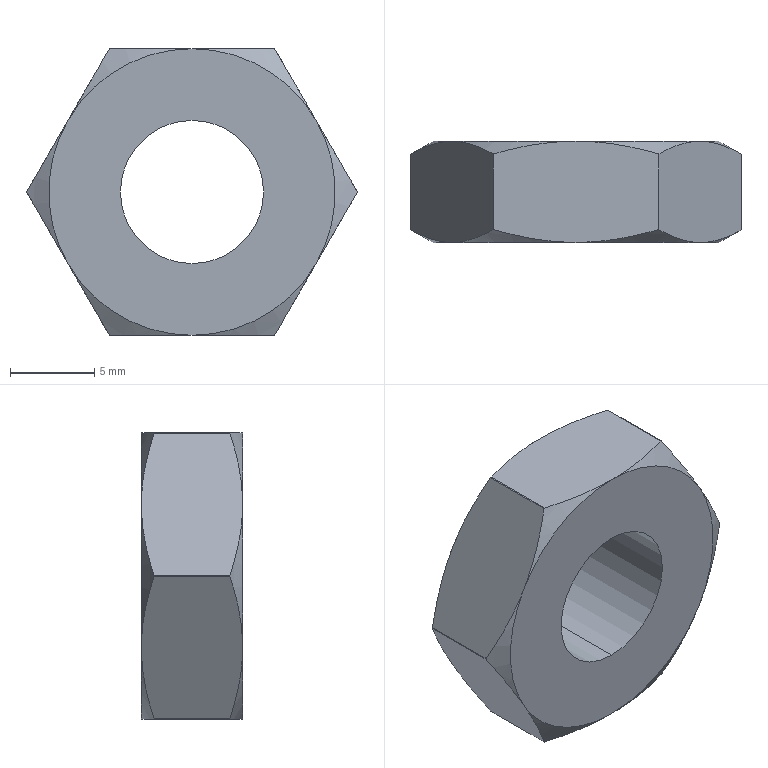Part | STEP file | 0229_Z_Cylinder_CG1BN25-50_4 | 1 solid | 28 faces | box 19.6 x 6 x 17 mm | volume 1151 mm3 | cone 12 | cylinder 8 | plane 8 | commonest cylinder face diameters 19.6 x6 8.5 x2